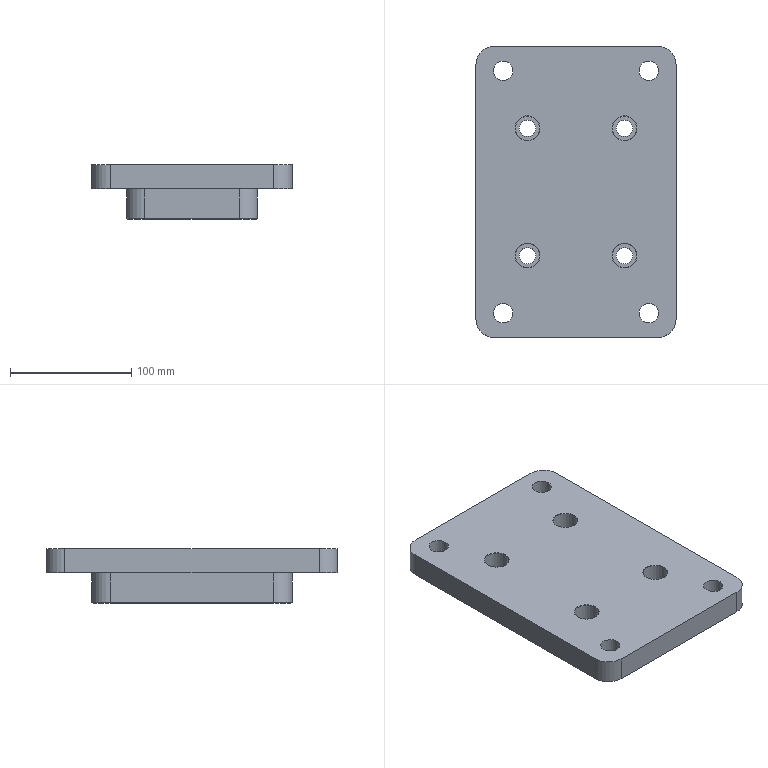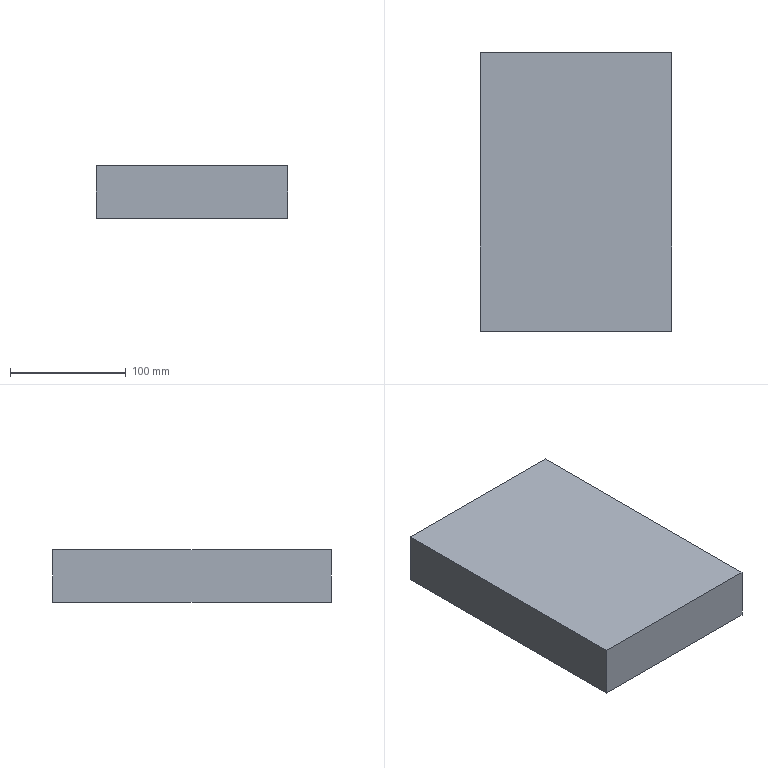CAM job | NX | 3-axis milling, drilling | part box 165 x 240 x 45 mm | stock box 165 x 240 x 45 mm
Tools:
number,name,description,diameter,corner_radius,flute_length,length,flutes
1,ZXZ,Milling Tool-5 Parameters,6.0,0.0,50.0,75.0,2
13,13.5ZT,Drilling Tool,13.5,0.0,35.0,50.0,2
11,D10JING,Milling Tool-5 Parameters,10.0,0.0,50.0,75.0,2
10,D10,Milling Tool-5 Parameters,10.0,0.0,50.0,75.0,2
7,D6A45,Milling Tool-5 Parameters,6.0,0.0,50.0,75.0,2
5,D25R0.5,Milling Tool-5 Parameters,25.0,0.5,50.0,75.0,2
Operations:
program,operation,operation_type,tool,method,geometry_group,spindle_rpm,surface_speed,feed_per_tooth,feed_cut,feed_plunge,cut_length_mm,path_length_mm,cut_time_min,machine_time_min
1,DRILLING,Operation,ZXZ,METHOD,A,5000.0,94.0,0.025,250.0,0.0,32.0,678.044,0.128,0.1926
1,DRILLING_COPY,Operation,13.5ZT,METHOD,A,2000.0,84.0,0.05,200.0,0.0,328.447,1270.937,1.642,1.736
1,ZLEVEL_PROFILE_1_COPY,ZLevelMilling,D10,METHOD,A,3200.0,100.0,0.3438,2200.0,100.0,16191.584,44548.187,7.36,10.195
1,HOLE_MILLING,CylinderMilling,D10,METHOD,A,3200.0,100.0,0.3438,2200.0,100.0,19405.67,20566.241,8.821,8.937
1,HOLE_MILLING_COPY,CylinderMilling,D10JING,METHOD,A,5000.0,157.0,0.12,1200.0,100.0,1085.655,2246.227,0.9047,1.021
1,ZLEVEL_PROFILE_1,ZLevelMilling,D10JING,METHOD,A,5000.0,157.0,0.125,1250.0,100.0,207.045,1187.045,0.1656,0.2636
1,PLANAR_MILL_COPY_COPY,PlanarMilling,D6A45,METHOD,A,7500.0,141.0,0.0833,1250.0,100.0,1255.451,2354.749,1.004,1.114
2,ZLEVEL_PROFILE_COPY,ZLevelMilling,D25R0.5,METHOD,B,2000.0,157.0,0.55,2200.0,1000.0,56037.113,56115.963,25.541,25.549
2,ZLEVEL_PROFILE_COPY_COPY_COPY,ZLevelMilling,D25R0.5,METHOD,B,2000.0,157.0,0.55,2200.0,1000.0,49345.521,49424.371,22.5,22.508
2,ZLEVEL_PROFILE_COPY_COPY,ZLevelMilling,D25R0.5,METHOD,B,2000.0,157.0,0.55,2200.0,1000.0,42720.844,42799.694,19.488,19.496
2,FLOOR_WALL,VolumeBased25DMillingOperation,D10JING,METHOD,B,5000.0,157.0,0.12,1200.0,500.0,5441.749,6000.444,4.422,4.478
2,PLANAR_MILL_COPY_COPY_COPY,PlanarMilling,D6A45,METHOD,B,7500.0,141.0,0.0833,1250.0,100.0,181.005,693.007,0.1448,0.196
2,PLANAR_MILL_COPY_COPY_COPY_COPY,PlanarMilling,D6A45,METHOD,B,7500.0,141.0,0.0833,1250.0,100.0,536.477,594.477,0.4292,0.435
2,PLANAR_MILL_COPY_COPY_COPY_COPY_1,PlanarMilling,D6A45,METHOD,B,7500.0,141.0,0.0833,1250.0,100.0,999.532,1997.141,0.7996,0.8994